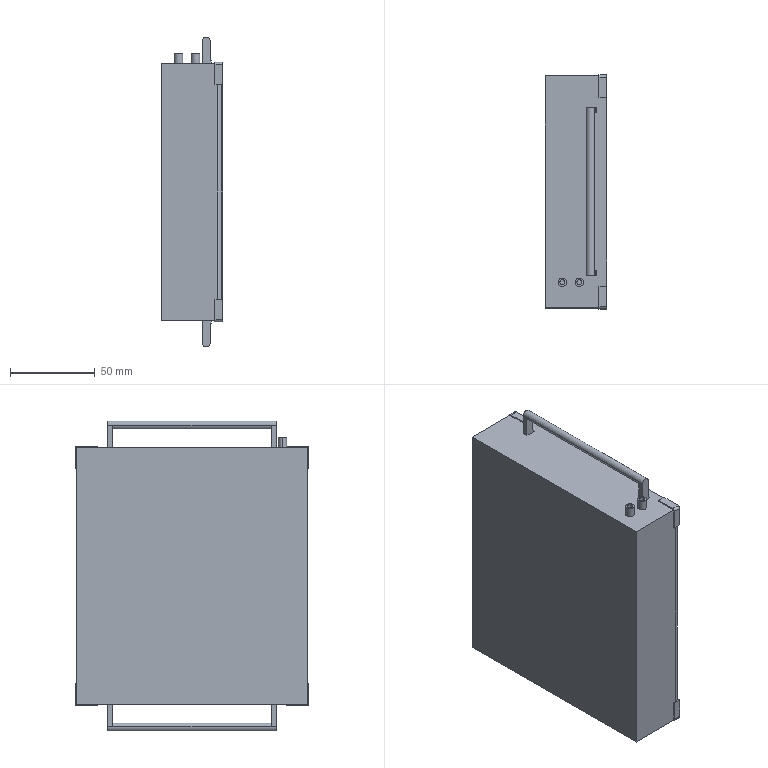Part | SolidWorks | features ICE 1, MBimport 1, Scale 1 | 1 solid | 119 faces | box 36 x 137.7 x 182.4 mm | volume 710177 mm3 | plane 81 | cylinder 38 | commonest cylinder face diameters 3 x12 4.5 x10 6 x8 4.8 x4 5 x4